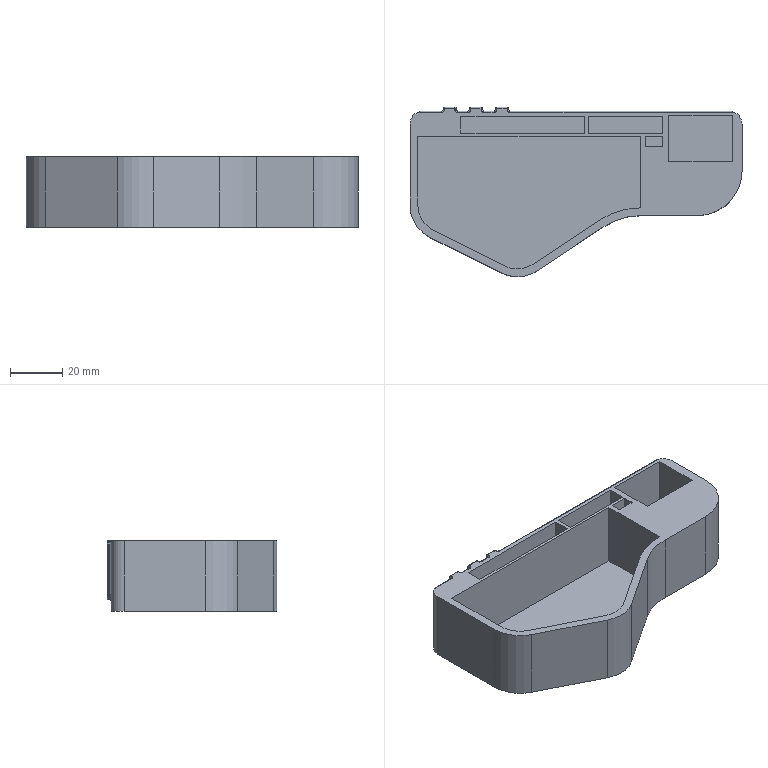Part | STEP file | DEWALT-DWE7492-B22 | 1 solid | 117 faces | box 126.934 x 64.887 x 27 mm | volume 57181 mm3 | cylinder 47 | plane 46 | torus 18 | sphere 6 | commonest cylinder face diameters 1 x32 4 x6 10 x2 21.631 x1 21.784 x1 27.631 x1